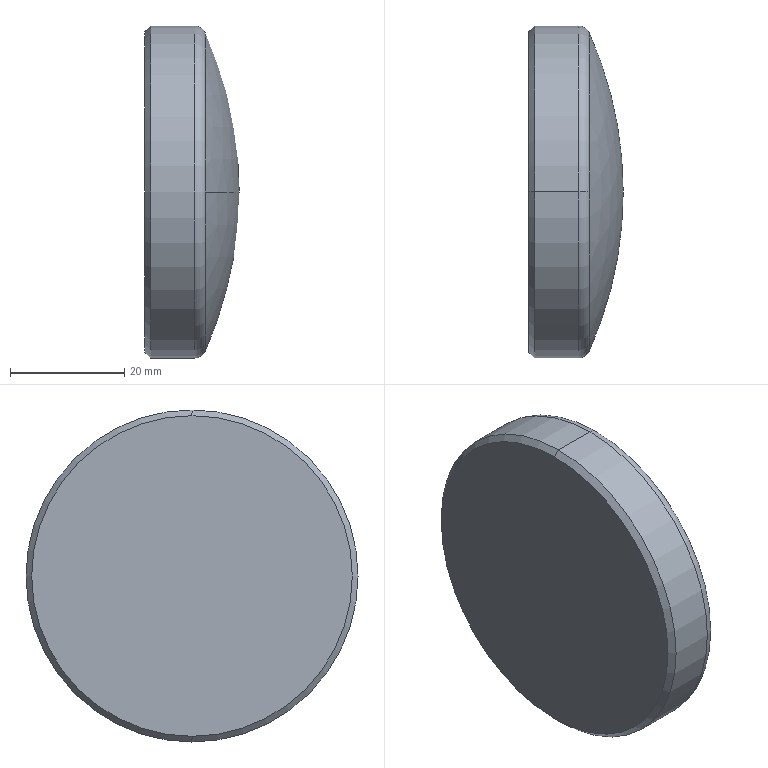Part | SolidWorks | features Chamfer 1, Fillet 1, Revolution 1 | 1 solid | 9 faces | box 16.494 x 58 x 58 mm | volume 35001 mm3 | cone 2 | torus 2 | sphere 2 | cylinder 2 | plane 1 | commonest cylinder face diameters 58 x2
STEP:
#1=CARTESIAN_POINT('',(0.,29.,28.));
#2=VERTEX_POINT('',#1);
#3=CARTESIAN_POINT('',(0.,29.,-28.));
#4=VERTEX_POINT('',#3);
#5=CARTESIAN_POINT('',(0.,29.,0.));
#6=DIRECTION('',(-1.,0.,0.));
#7=DIRECTION('',(0.,0.,1.));
#8=AXIS2_PLACEMENT_3D('',#5,#6,#7);
#9=CIRCLE('',#8,28.);
#10=EDGE_CURVE('',#2,#4,#9,.T.);
#11=ORIENTED_EDGE('',*,*,#10,.F.);
#12=CARTESIAN_POINT('',(1.,29.,29.));
#13=VERTEX_POINT('',#12);
#14=CARTESIAN_POINT('',(0.,29.,28.));
#15=DIRECTION('',(0.7071,0.,0.7071));
#16=VECTOR('',#15,1000.);
#17=LINE('',#14,#16);
#18=EDGE_CURVE('',#2,#13,#17,.T.);
#19=ORIENTED_EDGE('',*,*,#18,.T.);
#20=CARTESIAN_POINT('',(1.,29.,-29.));
#21=VERTEX_POINT('',#20);
#22=CARTESIAN_POINT('',(1.,29.,0.));
#23=DIRECTION('',(1.,0.,0.));
#24=DIRECTION('',(0.,0.,1.));
#25=AXIS2_PLACEMENT_3D('',#22,#23,#24);
#26=CIRCLE('',#25,29.);
#27=EDGE_CURVE('',#21,#13,#26,.T.);
#28=ORIENTED_EDGE('',*,*,#27,.F.);
#29=CARTESIAN_POINT('',(0.,29.,-28.));
#30=DIRECTION('',(0.7071,0.,-0.7071));
#31=VECTOR('',#30,1000.);
#32=LINE('',#29,#31);
#33=EDGE_CURVE('',#4,#21,#32,.T.);
#34=ORIENTED_EDGE('',*,*,#33,.F.);
#35=EDGE_LOOP('',(#11,#19,#28,#34));
#36=FACE_OUTER_BOUND('',#35,.T.);
#37=CARTESIAN_POINT('',(0.,29.,0.));
#38=DIRECTION('',(1.,0.,0.));
#39=DIRECTION('',(0.,0.,-1.));
#40=AXIS2_PLACEMENT_3D('',#37,#38,#39);
#41=CONICAL_SURFACE('',#40,28.,0.7854);
#42=ADVANCED_FACE('',(#36),#41,.T.);
#43=CARTESIAN_POINT('',(10.543,29.,-27.818));
#44=VERTEX_POINT('',#43);
#45=CARTESIAN_POINT('',(10.543,56.818,0.));
#46=VERTEX_POINT('',#45);
#47=CARTESIAN_POINT('',(10.543,29.,0.));
#48=DIRECTION('',(1.,0.,0.));
#49=DIRECTION('',(0.,0.,1.));
#50=AXIS2_PLACEMENT_3D('',#47,#48,#49);
#51=CIRCLE('',#50,27.818);
#52=EDGE_CURVE('',#44,#46,#51,.T.);
#53=ORIENTED_EDGE('',*,*,#52,.F.);
#54=CARTESIAN_POINT('',(8.718,29.,-29.));
#55=VERTEX_POINT('',#54);
#56=CARTESIAN_POINT('',(8.718,29.,-27.));
#57=DIRECTION('',(0.,1.,0.));
#58=DIRECTION('',(0.,0.,1.));
#59=AXIS2_PLACEMENT_3D('',#56,#57,#58);
#60=CIRCLE('',#59,2.);
#61=EDGE_CURVE('',#44,#55,#60,.T.);
#62=ORIENTED_EDGE('',*,*,#61,.T.);
#63=CARTESIAN_POINT('',(8.718,29.,29.));
#64=VERTEX_POINT('',#63);
#65=CARTESIAN_POINT('',(8.718,29.,0.));
#66=DIRECTION('',(-1.,0.,0.));
#67=DIRECTION('',(0.,0.,1.));
#68=AXIS2_PLACEMENT_3D('',#65,#66,#67);
#69=CIRCLE('',#68,29.);
#70=EDGE_CURVE('',#64,#55,#69,.T.);
#71=ORIENTED_EDGE('',*,*,#70,.F.);
#72=CARTESIAN_POINT('',(10.543,29.,27.818));
#73=VERTEX_POINT('',#72);
#74=CARTESIAN_POINT('',(8.718,29.,27.));
#75=DIRECTION('',(0.,-1.,0.));
#76=DIRECTION('',(0.,0.,-1.));
#77=AXIS2_PLACEMENT_3D('',#74,#75,#76);
#78=CIRCLE('',#77,2.);
#79=EDGE_CURVE('',#73,#64,#78,.T.);
#80=ORIENTED_EDGE('',*,*,#79,.F.);
#81=CARTESIAN_POINT('',(10.543,29.,0.));
#82=DIRECTION('',(1.,0.,0.));
#83=DIRECTION('',(0.,0.,1.));
#84=AXIS2_PLACEMENT_3D('',#81,#82,#83);
#85=CIRCLE('',#84,27.818);
#86=EDGE_CURVE('',#46,#73,#85,.T.);
#87=ORIENTED_EDGE('',*,*,#86,.F.);
#88=EDGE_LOOP('',(#53,#62,#71,#80,#87));
#89=FACE_OUTER_BOUND('',#88,.T.);
#90=CARTESIAN_POINT('',(8.718,29.,0.));
#91=DIRECTION('',(-1.,0.,0.));
#92=DIRECTION('',(0.,0.,1.));
#93=AXIS2_PLACEMENT_3D('',#90,#91,#92);
#94=TOROIDAL_SURFACE('',#93,27.,2.);
#95=ADVANCED_FACE('',(#89),#94,.T.);
#96=CARTESIAN_POINT('',(16.494,29.,0.));
#97=VERTEX_POINT('',#96);
#98=CARTESIAN_POINT('',(10.543,1.182,0.));
#99=VERTEX_POINT('',#98);
#100=CARTESIAN_POINT('',(-51.506,29.,0.));
#101=DIRECTION('',(0.,0.,-1.));
#102=DIRECTION('',(-1.,0.,0.));
#103=AXIS2_PLACEMENT_3D('',#100,#101,#102);
#104=CIRCLE('',#103,68.);
#105=EDGE_CURVE('',#97,#99,#104,.T.);
#106=ORIENTED_EDGE('',*,*,#105,.F.);
#107=CARTESIAN_POINT('',(-51.506,29.,0.));
#108=DIRECTION('',(0.,0.,1.));
#109=DIRECTION('',(0.,-1.,0.));
#110=AXIS2_PLACEMENT_3D('',#107,#108,#109);
#111=CIRCLE('',#110,68.);
#112=EDGE_CURVE('',#97,#46,#111,.T.);
#113=ORIENTED_EDGE('',*,*,#112,.T.);
#114=ORIENTED_EDGE('',*,*,#86,.T.);
#115=CARTESIAN_POINT('',(10.543,29.,0.));
#116=DIRECTION('',(1.,0.,0.));
#117=DIRECTION('',(0.,0.,1.));
#118=AXIS2_PLACEMENT_3D('',#115,#116,#117);
#119=CIRCLE('',#118,27.818);
#120=EDGE_CURVE('',#73,#99,#119,.T.);
#121=ORIENTED_EDGE('',*,*,#120,.T.);
#122=EDGE_LOOP('',(#106,#113,#114,#121));
#123=FACE_OUTER_BOUND('',#122,.T.);
#124=CARTESIAN_POINT('',(-51.506,29.,0.));
#125=DIRECTION('',(0.,0.,1.));
#126=DIRECTION('',(0.,-1.,0.));
#127=AXIS2_PLACEMENT_3D('',#124,#125,#126);
#128=SPHERICAL_SURFACE('',#127,68.);
#129=ADVANCED_FACE('',(#123),#128,.T.);
#130=ORIENTED_EDGE('',*,*,#70,.T.);
#131=CARTESIAN_POINT('',(-110.538,29.,-29.));
#132=DIRECTION('',(-1.,0.,0.));
#133=VECTOR('',#132,1000.);
#134=LINE('',#131,#133);
#135=EDGE_CURVE('',#55,#21,#134,.T.);
#136=ORIENTED_EDGE('',*,*,#135,.T.);
#137=ORIENTED_EDGE('',*,*,#27,.T.);
#138=CARTESIAN_POINT('',(-110.538,29.,29.));
#139=DIRECTION('',(-1.,0.,0.));
#140=VECTOR('',#139,1000.);
#141=LINE('',#138,#140);
#142=EDGE_CURVE('',#64,#13,#141,.T.);
#143=ORIENTED_EDGE('',*,*,#142,.F.);
#144=EDGE_LOOP('',(#130,#136,#137,#143));
#145=FACE_OUTER_BOUND('',#144,.T.);
#146=CARTESIAN_POINT('',(-110.538,29.,0.));
#147=DIRECTION('',(-1.,0.,0.));
#148=DIRECTION('',(0.,0.,1.));
#149=AXIS2_PLACEMENT_3D('',#146,#147,#148);
#150=CYLINDRICAL_SURFACE('',#149,29.);
#151=ADVANCED_FACE('',(#145),#150,.T.);
#152=CARTESIAN_POINT('',(0.,29.,0.));
#153=DIRECTION('',(-1.,0.,0.));
#154=DIRECTION('',(0.,0.,1.));
#155=AXIS2_PLACEMENT_3D('',#152,#153,#154);
#156=CIRCLE('',#155,28.);
#157=EDGE_CURVE('',#4,#2,#156,.T.);
#158=ORIENTED_EDGE('',*,*,#157,.T.);
#159=ORIENTED_EDGE('',*,*,#10,.T.);
#160=EDGE_LOOP('',(#158,#159));
#161=FACE_OUTER_BOUND('',#160,.T.);
#162=CARTESIAN_POINT('',(0.,0.,0.));
#163=DIRECTION('',(-1.,0.,0.));
#164=DIRECTION('',(0.,0.,1.));
#165=AXIS2_PLACEMENT_3D('',#162,#163,#164);
#166=PLANE('',#165);
#167=ADVANCED_FACE('',(#161),#166,.T.);
#168=ORIENTED_EDGE('',*,*,#135,.F.);
#169=CARTESIAN_POINT('',(8.718,29.,0.));
#170=DIRECTION('',(-1.,0.,0.));
#171=DIRECTION('',(0.,0.,1.));
#172=AXIS2_PLACEMENT_3D('',#169,#170,#171);
#173=CIRCLE('',#172,29.);
#174=EDGE_CURVE('',#55,#64,#173,.T.);
#175=ORIENTED_EDGE('',*,*,#174,.T.);
#176=ORIENTED_EDGE('',*,*,#142,.T.);
#177=CARTESIAN_POINT('',(1.,29.,0.));
#178=DIRECTION('',(1.,0.,0.));
#179=DIRECTION('',(0.,0.,1.));
#180=AXIS2_PLACEMENT_3D('',#177,#178,#179);
#181=CIRCLE('',#180,29.);
#182=EDGE_CURVE('',#13,#21,#181,.T.);
#183=ORIENTED_EDGE('',*,*,#182,.T.);
#184=EDGE_LOOP('',(#168,#175,#176,#183));
#185=FACE_OUTER_BOUND('',#184,.T.);
#186=CARTESIAN_POINT('',(-110.538,29.,0.));
#187=DIRECTION('',(-1.,0.,0.));
#188=DIRECTION('',(0.,0.,1.));
#189=AXIS2_PLACEMENT_3D('',#186,#187,#188);
#190=CYLINDRICAL_SURFACE('',#189,29.);
#191=ADVANCED_FACE('',(#185),#190,.T.);
#192=ORIENTED_EDGE('',*,*,#112,.F.);
#193=ORIENTED_EDGE('',*,*,#105,.T.);
#194=CARTESIAN_POINT('',(10.543,29.,0.));
#195=DIRECTION('',(1.,0.,0.));
#196=DIRECTION('',(0.,0.,1.));
#197=AXIS2_PLACEMENT_3D('',#194,#195,#196);
#198=CIRCLE('',#197,27.818);
#199=EDGE_CURVE('',#99,#44,#198,.T.);
#200=ORIENTED_EDGE('',*,*,#199,.T.);
#201=ORIENTED_EDGE('',*,*,#52,.T.);
#202=EDGE_LOOP('',(#192,#193,#200,#201));
#203=FACE_OUTER_BOUND('',#202,.T.);
#204=CARTESIAN_POINT('',(-51.506,29.,0.));
#205=DIRECTION('',(0.,0.,1.));
#206=DIRECTION('',(0.,-1.,0.));
#207=AXIS2_PLACEMENT_3D('',#204,#205,#206);
#208=SPHERICAL_SURFACE('',#207,68.);
#209=ADVANCED_FACE('',(#203),#208,.T.);
#210=ORIENTED_EDGE('',*,*,#61,.F.);
#211=ORIENTED_EDGE('',*,*,#199,.F.);
#212=ORIENTED_EDGE('',*,*,#120,.F.);
#213=ORIENTED_EDGE('',*,*,#79,.T.);
#214=ORIENTED_EDGE('',*,*,#174,.F.);
#215=EDGE_LOOP('',(#210,#211,#212,#213,#214));
#216=FACE_OUTER_BOUND('',#215,.T.);
#217=CARTESIAN_POINT('',(8.718,29.,0.));
#218=DIRECTION('',(-1.,0.,0.));
#219=DIRECTION('',(0.,0.,1.));
#220=AXIS2_PLACEMENT_3D('',#217,#218,#219);
#221=TOROIDAL_SURFACE('',#220,27.,2.);
#222=ADVANCED_FACE('',(#216),#221,.T.);
#223=ORIENTED_EDGE('',*,*,#18,.F.);
#224=ORIENTED_EDGE('',*,*,#157,.F.);
#225=ORIENTED_EDGE('',*,*,#33,.T.);
#226=ORIENTED_EDGE('',*,*,#182,.F.);
#227=EDGE_LOOP('',(#223,#224,#225,#226));
#228=FACE_OUTER_BOUND('',#227,.T.);
#229=CARTESIAN_POINT('',(0.,29.,0.));
#230=DIRECTION('',(1.,0.,0.));
#231=DIRECTION('',(0.,0.,-1.));
#232=AXIS2_PLACEMENT_3D('',#229,#230,#231);
#233=CONICAL_SURFACE('',#232,28.,0.7854);
#234=ADVANCED_FACE('',(#228),#233,.T.);
#235=CLOSED_SHELL('',(#42,#95,#129,#151,#167,#191,#209,#222,#234));
#236=MANIFOLD_SOLID_BREP('',#235);
#237=CARTESIAN_POINT('',(0.,0.,0.));
#238=DIRECTION('',(0.,0.,1.));
#239=DIRECTION('',(1.,0.,0.));
#240=AXIS2_PLACEMENT_3D('',#237,#238,#239);
#241=(LENGTH_UNIT()NAMED_UNIT(*)SI_UNIT(.MILLI.,.METRE.));
#242=UNCERTAINTY_MEASURE_WITH_UNIT(LENGTH_MEASURE(0.00001),#241,'','');
#243=(NAMED_UNIT(*)PLANE_ANGLE_UNIT()SI_UNIT($,.RADIAN.));
#244=(NAMED_UNIT(*)SI_UNIT($,.STERADIAN.)SOLID_ANGLE_UNIT());
#245=(GEOMETRIC_REPRESENTATION_CONTEXT(3)GLOBAL_UNCERTAINTY_ASSIGNED_CONTEXT((#242))GLOBAL_UNIT_ASSIGNED_CONTEXT((#241,#243,#244))REPRESENTATION_CONTEXT('',''));
#246=ADVANCED_BREP_SHAPE_REPRESENTATION('',(#236,#240),#245);